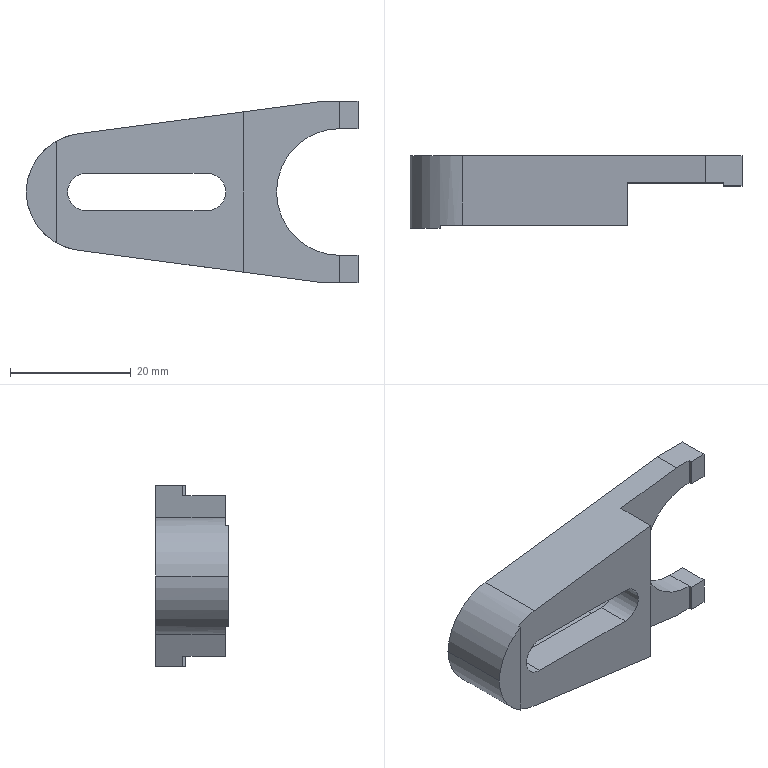Part | SolidWorks | features ICE 4, Extrusion 1, Fillet 1 | 1 solid | 33 faces | box 54.997 x 12 x 30 mm | volume 7361 mm3 | plane 23 | cylinder 10 | commonest cylinder face diameters 6.2 x3 11 x3 20 x2 21 x2
STEP:
#1=CARTESIAN_POINT('',(-50.5,-6.,15.));
#2=VERTEX_POINT('',#1);
#3=CARTESIAN_POINT('',(-45.,-6.,20.5));
#4=VERTEX_POINT('',#3);
#5=CARTESIAN_POINT('',(-45.,-6.,15.));
#6=DIRECTION('',(0.,1.,0.));
#7=DIRECTION('',(-1.,0.,0.));
#8=AXIS2_PLACEMENT_3D('',#5,#6,#7);
#9=CIRCLE('',#8,5.5);
#10=EDGE_CURVE('',#2,#4,#9,.T.);
#11=ORIENTED_EDGE('',*,*,#10,.F.);
#12=CARTESIAN_POINT('',(-50.5,0.,15.));
#13=VERTEX_POINT('',#12);
#14=CARTESIAN_POINT('',(-50.5,-6.,15.));
#15=DIRECTION('',(0.,1.,0.));
#16=VECTOR('',#15,1000.);
#17=LINE('',#14,#16);
#18=EDGE_CURVE('',#2,#13,#17,.T.);
#19=ORIENTED_EDGE('',*,*,#18,.T.);
#20=CARTESIAN_POINT('',(-45.,0.,20.5));
#21=VERTEX_POINT('',#20);
#22=CARTESIAN_POINT('',(-45.,0.,15.));
#23=DIRECTION('',(0.,1.,0.));
#24=DIRECTION('',(-1.,0.,0.));
#25=AXIS2_PLACEMENT_3D('',#22,#23,#24);
#26=CIRCLE('',#25,5.5);
#27=EDGE_CURVE('',#13,#21,#26,.T.);
#28=ORIENTED_EDGE('',*,*,#27,.T.);
#29=CARTESIAN_POINT('',(-45.,-6.,20.5));
#30=DIRECTION('',(0.,1.,0.));
#31=VECTOR('',#30,1000.);
#32=LINE('',#29,#31);
#33=EDGE_CURVE('',#4,#21,#32,.T.);
#34=ORIENTED_EDGE('',*,*,#33,.F.);
#35=EDGE_LOOP('',(#11,#19,#28,#34));
#36=FACE_OUTER_BOUND('',#35,.T.);
#37=CARTESIAN_POINT('',(-45.,-6.,15.));
#38=DIRECTION('',(0.,1.,0.));
#39=DIRECTION('',(-1.,0.,0.));
#40=AXIS2_PLACEMENT_3D('',#37,#38,#39);
#41=CYLINDRICAL_SURFACE('',#40,5.5);
#42=ADVANCED_FACE('',(#36),#41,.F.);
#43=CARTESIAN_POINT('',(-13.5,-4.5,15.));
#44=VERTEX_POINT('',#43);
#45=CARTESIAN_POINT('',(-3.,-4.5,25.5));
#46=VERTEX_POINT('',#45);
#47=CARTESIAN_POINT('',(-3.,-4.5,15.));
#48=DIRECTION('',(0.,1.,0.));
#49=DIRECTION('',(-1.,0.,0.));
#50=AXIS2_PLACEMENT_3D('',#47,#48,#49);
#51=CIRCLE('',#50,10.5);
#52=EDGE_CURVE('',#44,#46,#51,.T.);
#53=ORIENTED_EDGE('',*,*,#52,.F.);
#54=CARTESIAN_POINT('',(-13.5,0.,15.));
#55=VERTEX_POINT('',#54);
#56=CARTESIAN_POINT('',(-13.5,-12.,15.));
#57=DIRECTION('',(0.,1.,0.));
#58=VECTOR('',#57,1000.);
#59=LINE('',#56,#58);
#60=EDGE_CURVE('',#44,#55,#59,.T.);
#61=ORIENTED_EDGE('',*,*,#60,.T.);
#62=CARTESIAN_POINT('',(-3.,0.,25.5));
#63=VERTEX_POINT('',#62);
#64=CARTESIAN_POINT('',(-3.,0.,15.));
#65=DIRECTION('',(0.,1.,0.));
#66=DIRECTION('',(-1.,0.,0.));
#67=AXIS2_PLACEMENT_3D('',#64,#65,#66);
#68=CIRCLE('',#67,10.5);
#69=EDGE_CURVE('',#55,#63,#68,.T.);
#70=ORIENTED_EDGE('',*,*,#69,.T.);
#71=CARTESIAN_POINT('',(-3.,-12.,25.5));
#72=DIRECTION('',(0.,1.,0.));
#73=VECTOR('',#72,1000.);
#74=LINE('',#71,#73);
#75=EDGE_CURVE('',#46,#63,#74,.T.);
#76=ORIENTED_EDGE('',*,*,#75,.F.);
#77=EDGE_LOOP('',(#53,#61,#70,#76));
#78=FACE_OUTER_BOUND('',#77,.T.);
#79=CARTESIAN_POINT('',(-3.,-12.,15.));
#80=DIRECTION('',(0.,1.,0.));
#81=DIRECTION('',(-1.,0.,0.));
#82=AXIS2_PLACEMENT_3D('',#79,#80,#81);
#83=CYLINDRICAL_SURFACE('',#82,10.5);
#84=ADVANCED_FACE('',(#78),#83,.F.);
#85=CARTESIAN_POINT('',(-48.1,-11.5,15.));
#86=VERTEX_POINT('',#85);
#87=CARTESIAN_POINT('',(-45.,-11.5,18.1));
#88=VERTEX_POINT('',#87);
#89=CARTESIAN_POINT('',(-45.,-11.5,15.));
#90=DIRECTION('',(0.,1.,0.));
#91=DIRECTION('',(0.,0.,1.));
#92=AXIS2_PLACEMENT_3D('',#89,#90,#91);
#93=CIRCLE('',#92,3.1);
#94=EDGE_CURVE('',#86,#88,#93,.T.);
#95=ORIENTED_EDGE('',*,*,#94,.F.);
#96=CARTESIAN_POINT('',(-48.1,-6.,15.));
#97=VERTEX_POINT('',#96);
#98=CARTESIAN_POINT('',(-48.1,-12.,15.));
#99=DIRECTION('',(0.,1.,0.));
#100=VECTOR('',#99,1000.);
#101=LINE('',#98,#100);
#102=EDGE_CURVE('',#86,#97,#101,.T.);
#103=ORIENTED_EDGE('',*,*,#102,.T.);
#104=CARTESIAN_POINT('',(-45.,-6.,18.1));
#105=VERTEX_POINT('',#104);
#106=CARTESIAN_POINT('',(-45.,-6.,15.));
#107=DIRECTION('',(0.,-1.,0.));
#108=DIRECTION('',(-1.,0.,0.));
#109=AXIS2_PLACEMENT_3D('',#106,#107,#108);
#110=CIRCLE('',#109,3.1);
#111=EDGE_CURVE('',#105,#97,#110,.T.);
#112=ORIENTED_EDGE('',*,*,#111,.F.);
#113=CARTESIAN_POINT('',(-45.,-12.,18.1));
#114=DIRECTION('',(0.,1.,0.));
#115=VECTOR('',#114,1000.);
#116=LINE('',#113,#115);
#117=EDGE_CURVE('',#88,#105,#116,.T.);
#118=ORIENTED_EDGE('',*,*,#117,.F.);
#119=EDGE_LOOP('',(#95,#103,#112,#118));
#120=FACE_OUTER_BOUND('',#119,.T.);
#121=CARTESIAN_POINT('',(-45.,-12.,15.));
#122=DIRECTION('',(0.,1.,0.));
#123=DIRECTION('',(-1.,0.,0.));
#124=AXIS2_PLACEMENT_3D('',#121,#122,#123);
#125=CYLINDRICAL_SURFACE('',#124,3.1);
#126=ADVANCED_FACE('',(#120),#125,.F.);
#127=ORIENTED_EDGE('',*,*,#102,.F.);
#128=CARTESIAN_POINT('',(-45.,-11.5,11.9));
#129=VERTEX_POINT('',#128);
#130=CARTESIAN_POINT('',(-45.,-11.5,15.));
#131=DIRECTION('',(0.,1.,0.));
#132=DIRECTION('',(0.,0.,1.));
#133=AXIS2_PLACEMENT_3D('',#130,#131,#132);
#134=CIRCLE('',#133,3.1);
#135=EDGE_CURVE('',#129,#86,#134,.T.);
#136=ORIENTED_EDGE('',*,*,#135,.F.);
#137=CARTESIAN_POINT('',(-45.,-6.,11.9));
#138=VERTEX_POINT('',#137);
#139=CARTESIAN_POINT('',(-45.,-12.,11.9));
#140=DIRECTION('',(0.,1.,0.));
#141=VECTOR('',#140,1000.);
#142=LINE('',#139,#141);
#143=EDGE_CURVE('',#129,#138,#142,.T.);
#144=ORIENTED_EDGE('',*,*,#143,.T.);
#145=CARTESIAN_POINT('',(-45.,-6.,15.));
#146=DIRECTION('',(0.,-1.,0.));
#147=DIRECTION('',(-1.,0.,0.));
#148=AXIS2_PLACEMENT_3D('',#145,#146,#147);
#149=CIRCLE('',#148,3.1);
#150=EDGE_CURVE('',#97,#138,#149,.T.);
#151=ORIENTED_EDGE('',*,*,#150,.F.);
#152=EDGE_LOOP('',(#127,#136,#144,#151));
#153=FACE_OUTER_BOUND('',#152,.T.);
#154=CARTESIAN_POINT('',(-45.,-12.,15.));
#155=DIRECTION('',(0.,1.,0.));
#156=DIRECTION('',(-1.,0.,0.));
#157=AXIS2_PLACEMENT_3D('',#154,#155,#156);
#158=CYLINDRICAL_SURFACE('',#157,3.1);
#159=ADVANCED_FACE('',(#153),#158,.F.);
#160=CARTESIAN_POINT('',(-25.,-6.,11.9));
#161=VERTEX_POINT('',#160);
#162=CARTESIAN_POINT('',(-45.,-6.,11.9));
#163=DIRECTION('',(1.,0.,0.));
#164=VECTOR('',#163,1000.);
#165=LINE('',#162,#164);
#166=EDGE_CURVE('',#138,#161,#165,.T.);
#167=ORIENTED_EDGE('',*,*,#166,.F.);
#168=ORIENTED_EDGE('',*,*,#143,.F.);
#169=CARTESIAN_POINT('',(-25.,-11.5,11.9));
#170=VERTEX_POINT('',#169);
#171=CARTESIAN_POINT('',(-50.,-11.5,11.9));
#172=DIRECTION('',(-1.,0.,0.));
#173=VECTOR('',#172,1000.);
#174=LINE('',#171,#173);
#175=EDGE_CURVE('',#170,#129,#174,.T.);
#176=ORIENTED_EDGE('',*,*,#175,.F.);
#177=CARTESIAN_POINT('',(-25.,-12.,11.9));
#178=DIRECTION('',(0.,1.,0.));
#179=VECTOR('',#178,1000.);
#180=LINE('',#177,#179);
#181=EDGE_CURVE('',#170,#161,#180,.T.);
#182=ORIENTED_EDGE('',*,*,#181,.T.);
#183=EDGE_LOOP('',(#167,#168,#176,#182));
#184=FACE_OUTER_BOUND('',#183,.T.);
#185=CARTESIAN_POINT('',(-45.,-12.,11.9));
#186=DIRECTION('',(0.,0.,-1.));
#187=DIRECTION('',(-1.,0.,0.));
#188=AXIS2_PLACEMENT_3D('',#185,#186,#187);
#189=PLANE('',#188);
#190=ADVANCED_FACE('',(#184),#189,.F.);
#191=CARTESIAN_POINT('',(-25.,-6.,18.1));
#192=VERTEX_POINT('',#191);
#193=CARTESIAN_POINT('',(-25.,-6.,15.));
#194=DIRECTION('',(0.,-1.,0.));
#195=DIRECTION('',(-1.,0.,0.));
#196=AXIS2_PLACEMENT_3D('',#193,#194,#195);
#197=CIRCLE('',#196,3.1);
#198=EDGE_CURVE('',#161,#192,#197,.T.);
#199=ORIENTED_EDGE('',*,*,#198,.F.);
#200=ORIENTED_EDGE('',*,*,#181,.F.);
#201=CARTESIAN_POINT('',(-25.,-11.5,18.1));
#202=VERTEX_POINT('',#201);
#203=CARTESIAN_POINT('',(-25.,-11.5,15.));
#204=DIRECTION('',(0.,1.,0.));
#205=DIRECTION('',(0.,0.,1.));
#206=AXIS2_PLACEMENT_3D('',#203,#204,#205);
#207=CIRCLE('',#206,3.1);
#208=EDGE_CURVE('',#202,#170,#207,.T.);
#209=ORIENTED_EDGE('',*,*,#208,.F.);
#210=CARTESIAN_POINT('',(-25.,-12.,18.1));
#211=DIRECTION('',(0.,1.,0.));
#212=VECTOR('',#211,1000.);
#213=LINE('',#210,#212);
#214=EDGE_CURVE('',#202,#192,#213,.T.);
#215=ORIENTED_EDGE('',*,*,#214,.T.);
#216=EDGE_LOOP('',(#199,#200,#209,#215));
#217=FACE_OUTER_BOUND('',#216,.T.);
#218=CARTESIAN_POINT('',(-25.,-12.,15.));
#219=DIRECTION('',(0.,1.,0.));
#220=DIRECTION('',(-1.,0.,0.));
#221=AXIS2_PLACEMENT_3D('',#218,#219,#220);
#222=CYLINDRICAL_SURFACE('',#221,3.1);
#223=ADVANCED_FACE('',(#217),#222,.F.);
#224=CARTESIAN_POINT('',(-45.,-6.,18.1));
#225=DIRECTION('',(-1.,0.,0.));
#226=VECTOR('',#225,1000.);
#227=LINE('',#224,#226);
#228=EDGE_CURVE('',#192,#105,#227,.T.);
#229=ORIENTED_EDGE('',*,*,#228,.F.);
#230=ORIENTED_EDGE('',*,*,#214,.F.);
#231=CARTESIAN_POINT('',(-50.,-11.5,18.1));
#232=DIRECTION('',(1.,0.,0.));
#233=VECTOR('',#232,1000.);
#234=LINE('',#231,#233);
#235=EDGE_CURVE('',#88,#202,#234,.T.);
#236=ORIENTED_EDGE('',*,*,#235,.F.);
#237=ORIENTED_EDGE('',*,*,#117,.T.);
#238=EDGE_LOOP('',(#229,#230,#236,#237));
#239=FACE_OUTER_BOUND('',#238,.T.);
#240=CARTESIAN_POINT('',(-45.,-12.,18.1));
#241=DIRECTION('',(0.,0.,1.));
#242=DIRECTION('',(1.,0.,0.));
#243=AXIS2_PLACEMENT_3D('',#240,#241,#242);
#244=PLANE('',#243);
#245=ADVANCED_FACE('',(#239),#244,.F.);
#246=CARTESIAN_POINT('',(-3.,-4.5,4.5));
#247=VERTEX_POINT('',#246);
#248=CARTESIAN_POINT('',(-3.,-4.5,0.));
#249=VERTEX_POINT('',#248);
#250=CARTESIAN_POINT('',(-3.,-4.5,4.5));
#251=DIRECTION('',(0.,0.,-1.));
#252=VECTOR('',#251,1000.);
#253=LINE('',#250,#252);
#254=EDGE_CURVE('',#247,#249,#253,.T.);
#255=ORIENTED_EDGE('',*,*,#254,.F.);
#256=CARTESIAN_POINT('',(-3.,-4.5,15.));
#257=DIRECTION('',(0.,1.,0.));
#258=DIRECTION('',(-1.,0.,0.));
#259=AXIS2_PLACEMENT_3D('',#256,#257,#258);
#260=CIRCLE('',#259,10.5);
#261=EDGE_CURVE('',#247,#44,#260,.T.);
#262=ORIENTED_EDGE('',*,*,#261,.T.);
#263=ORIENTED_EDGE('',*,*,#52,.T.);
#264=CARTESIAN_POINT('',(-3.,-4.5,30.));
#265=VERTEX_POINT('',#264);
#266=CARTESIAN_POINT('',(-3.,-4.5,25.5));
#267=DIRECTION('',(0.,0.,-1.));
#268=VECTOR('',#267,1000.);
#269=LINE('',#266,#268);
#270=EDGE_CURVE('',#265,#46,#269,.T.);
#271=ORIENTED_EDGE('',*,*,#270,.F.);
#272=CARTESIAN_POINT('',(-6.,-4.5,30.));
#273=VERTEX_POINT('',#272);
#274=CARTESIAN_POINT('',(0.,-4.5,30.));
#275=DIRECTION('',(1.,0.,0.));
#276=VECTOR('',#275,1000.);
#277=LINE('',#274,#276);
#278=EDGE_CURVE('',#273,#265,#277,.T.);
#279=ORIENTED_EDGE('',*,*,#278,.F.);
#280=CARTESIAN_POINT('',(-19.,-4.5,28.276));
#281=VERTEX_POINT('',#280);
#282=CARTESIAN_POINT('',(-0.1038,-4.5,30.782));
#283=DIRECTION('',(-0.9913,0.,-0.1315));
#284=VECTOR('',#283,1000.);
#285=LINE('',#282,#284);
#286=EDGE_CURVE('',#273,#281,#285,.T.);
#287=ORIENTED_EDGE('',*,*,#286,.T.);
#288=CARTESIAN_POINT('',(-19.,-4.5,1.724));
#289=VERTEX_POINT('',#288);
#290=CARTESIAN_POINT('',(-19.,-4.5,30.));
#291=DIRECTION('',(0.,0.,-1.));
#292=VECTOR('',#291,1000.);
#293=LINE('',#290,#292);
#294=EDGE_CURVE('',#281,#289,#293,.T.);
#295=ORIENTED_EDGE('',*,*,#294,.T.);
#296=CARTESIAN_POINT('',(-6.,-4.5,0.));
#297=VERTEX_POINT('',#296);
#298=CARTESIAN_POINT('',(-4.015,-4.5,-0.2634));
#299=DIRECTION('',(0.9913,0.,-0.1315));
#300=VECTOR('',#299,1000.);
#301=LINE('',#298,#300);
#302=EDGE_CURVE('',#289,#297,#301,.T.);
#303=ORIENTED_EDGE('',*,*,#302,.T.);
#304=CARTESIAN_POINT('',(0.,-4.5,0.));
#305=DIRECTION('',(1.,0.,0.));
#306=VECTOR('',#305,1000.);
#307=LINE('',#304,#306);
#308=EDGE_CURVE('',#297,#249,#307,.T.);
#309=ORIENTED_EDGE('',*,*,#308,.T.);
#310=EDGE_LOOP('',(#255,#262,#263,#271,#279,#287,#295,#303,#309));
#311=FACE_OUTER_BOUND('',#310,.T.);
#312=CARTESIAN_POINT('',(0.,-4.5,30.));
#313=DIRECTION('',(0.,1.,0.));
#314=DIRECTION('',(-1.,0.,0.));
#315=AXIS2_PLACEMENT_3D('',#312,#313,#314);
#316=PLANE('',#315);
#317=ADVANCED_FACE('',(#311),#316,.F.);
#318=CARTESIAN_POINT('',(0.,-5.,30.));
#319=VERTEX_POINT('',#318);
#320=CARTESIAN_POINT('',(0.,0.,30.));
#321=VERTEX_POINT('',#320);
#322=CARTESIAN_POINT('',(0.,0.,30.));
#323=DIRECTION('',(0.,1.,0.));
#324=VECTOR('',#323,1000.);
#325=LINE('',#322,#324);
#326=EDGE_CURVE('',#319,#321,#325,.T.);
#327=ORIENTED_EDGE('',*,*,#326,.F.);
#328=CARTESIAN_POINT('',(0.,-5.,25.5));
#329=VERTEX_POINT('',#328);
#330=CARTESIAN_POINT('',(0.,-5.,25.5));
#331=DIRECTION('',(0.,0.,1.));
#332=VECTOR('',#331,1000.);
#333=LINE('',#330,#332);
#334=EDGE_CURVE('',#329,#319,#333,.T.);
#335=ORIENTED_EDGE('',*,*,#334,.F.);
#336=CARTESIAN_POINT('',(0.,0.,25.5));
#337=VERTEX_POINT('',#336);
#338=CARTESIAN_POINT('',(0.,0.,25.5));
#339=DIRECTION('',(0.,1.,0.));
#340=VECTOR('',#339,1000.);
#341=LINE('',#338,#340);
#342=EDGE_CURVE('',#329,#337,#341,.T.);
#343=ORIENTED_EDGE('',*,*,#342,.T.);
#344=CARTESIAN_POINT('',(0.,0.,30.));
#345=DIRECTION('',(0.,0.,-1.));
#346=VECTOR('',#345,1000.);
#347=LINE('',#344,#346);
#348=EDGE_CURVE('',#321,#337,#347,.T.);
#349=ORIENTED_EDGE('',*,*,#348,.F.);
#350=EDGE_LOOP('',(#327,#335,#343,#349));
#351=FACE_OUTER_BOUND('',#350,.T.);
#352=CARTESIAN_POINT('',(0.,0.,30.));
#353=DIRECTION('',(-1.,0.,0.));
#354=DIRECTION('',(0.,-1.,0.));
#355=AXIS2_PLACEMENT_3D('',#352,#353,#354);
#356=PLANE('',#355);
#357=ADVANCED_FACE('',(#351),#356,.F.);
#358=CARTESIAN_POINT('',(0.,0.,4.5));
#359=VERTEX_POINT('',#358);
#360=CARTESIAN_POINT('',(0.,0.,0.));
#361=VERTEX_POINT('',#360);
#362=CARTESIAN_POINT('',(0.,0.,30.));
#363=DIRECTION('',(0.,0.,-1.));
#364=VECTOR('',#363,1000.);
#365=LINE('',#362,#364);
#366=EDGE_CURVE('',#359,#361,#365,.T.);
#367=ORIENTED_EDGE('',*,*,#366,.F.);
#368=CARTESIAN_POINT('',(0.,-5.,4.5));
#369=VERTEX_POINT('',#368);
#370=CARTESIAN_POINT('',(0.,0.,4.5));
#371=DIRECTION('',(0.,-1.,0.));
#372=VECTOR('',#371,1000.);
#373=LINE('',#370,#372);
#374=EDGE_CURVE('',#359,#369,#373,.T.);
#375=ORIENTED_EDGE('',*,*,#374,.T.);
#376=CARTESIAN_POINT('',(0.,-5.,0.));
#377=VERTEX_POINT('',#376);
#378=CARTESIAN_POINT('',(0.,-5.,4.5));
#379=DIRECTION('',(0.,0.,1.));
#380=VECTOR('',#379,1000.);
#381=LINE('',#378,#380);
#382=EDGE_CURVE('',#377,#369,#381,.T.);
#383=ORIENTED_EDGE('',*,*,#382,.F.);
#384=CARTESIAN_POINT('',(0.,0.,0.));
#385=DIRECTION('',(0.,1.,0.));
#386=VECTOR('',#385,1000.);
#387=LINE('',#384,#386);
#388=EDGE_CURVE('',#377,#361,#387,.T.);
#389=ORIENTED_EDGE('',*,*,#388,.T.);
#390=EDGE_LOOP('',(#367,#375,#383,#389));
#391=FACE_OUTER_BOUND('',#390,.T.);
#392=CARTESIAN_POINT('',(0.,0.,30.));
#393=DIRECTION('',(-1.,0.,0.));
#394=DIRECTION('',(0.,-1.,0.));
#395=AXIS2_PLACEMENT_3D('',#392,#393,#394);
#396=PLANE('',#395);
#397=ADVANCED_FACE('',(#391),#396,.F.);
#398=CARTESIAN_POINT('',(-25.,0.,20.5));
#399=VERTEX_POINT('',#398);
#400=CARTESIAN_POINT('',(-45.,0.,20.5));
#401=DIRECTION('',(1.,0.,0.));
#402=VECTOR('',#401,1000.);
#403=LINE('',#400,#402);
#404=EDGE_CURVE('',#21,#399,#403,.T.);
#405=ORIENTED_EDGE('',*,*,#404,.F.);
#406=ORIENTED_EDGE('',*,*,#27,.F.);
#407=CARTESIAN_POINT('',(-45.,0.,9.5));
#408=VERTEX_POINT('',#407);
#409=CARTESIAN_POINT('',(-45.,0.,15.));
#410=DIRECTION('',(0.,1.,0.));
#411=DIRECTION('',(-1.,0.,0.));
#412=AXIS2_PLACEMENT_3D('',#409,#410,#411);
#413=CIRCLE('',#412,5.5);
#414=EDGE_CURVE('',#408,#13,#413,.T.);
#415=ORIENTED_EDGE('',*,*,#414,.F.);
#416=CARTESIAN_POINT('',(-25.,0.,9.5));
#417=VERTEX_POINT('',#416);
#418=CARTESIAN_POINT('',(-45.,0.,9.5));
#419=DIRECTION('',(-1.,0.,0.));
#420=VECTOR('',#419,1000.);
#421=LINE('',#418,#420);
#422=EDGE_CURVE('',#417,#408,#421,.T.);
#423=ORIENTED_EDGE('',*,*,#422,.F.);
#424=CARTESIAN_POINT('',(-25.,0.,15.));
#425=DIRECTION('',(0.,1.,0.));
#426=DIRECTION('',(-1.,0.,0.));
#427=AXIS2_PLACEMENT_3D('',#424,#425,#426);
#428=CIRCLE('',#427,5.5);
#429=EDGE_CURVE('',#399,#417,#428,.T.);
#430=ORIENTED_EDGE('',*,*,#429,.F.);
#431=EDGE_LOOP('',(#405,#406,#415,#423,#430));
#432=FACE_BOUND('',#431,.T.);
#433=CARTESIAN_POINT('',(-46.315,0.,5.348));
#434=VERTEX_POINT('',#433);
#435=CARTESIAN_POINT('',(-6.,0.,0.));
#436=VERTEX_POINT('',#435);
#437=CARTESIAN_POINT('',(-6.,0.,0.));
#438=DIRECTION('',(0.9913,0.,-0.1315));
#439=VECTOR('',#438,1000.);
#440=LINE('',#437,#439);
#441=EDGE_CURVE('',#434,#436,#440,.T.);
#442=ORIENTED_EDGE('',*,*,#441,.F.);
#443=CARTESIAN_POINT('',(-54.997,0.,15.));
#444=VERTEX_POINT('',#443);
#445=CARTESIAN_POINT('',(-45.,0.,15.261));
#446=DIRECTION('',(0.,1.,0.));
#447=DIRECTION('',(1.,0.,0.));
#448=AXIS2_PLACEMENT_3D('',#445,#446,#447);
#449=CIRCLE('',#448,10.);
#450=EDGE_CURVE('',#434,#444,#449,.T.);
#451=ORIENTED_EDGE('',*,*,#450,.T.);
#452=CARTESIAN_POINT('',(-46.315,0.,24.652));
#453=VERTEX_POINT('',#452);
#454=CARTESIAN_POINT('',(-45.,0.,14.739));
#455=DIRECTION('',(0.,1.,0.));
#456=DIRECTION('',(1.,0.,0.));
#457=AXIS2_PLACEMENT_3D('',#454,#455,#456);
#458=CIRCLE('',#457,10.);
#459=EDGE_CURVE('',#444,#453,#458,.T.);
#460=ORIENTED_EDGE('',*,*,#459,.T.);
#461=CARTESIAN_POINT('',(-6.,0.,30.));
#462=VERTEX_POINT('',#461);
#463=CARTESIAN_POINT('',(-55.,0.,23.5));
#464=DIRECTION('',(-0.9913,0.,-0.1315));
#465=VECTOR('',#464,1000.);
#466=LINE('',#463,#465);
#467=EDGE_CURVE('',#462,#453,#466,.T.);
#468=ORIENTED_EDGE('',*,*,#467,.F.);
#469=CARTESIAN_POINT('',(0.,0.,30.));
#470=DIRECTION('',(-1.,0.,0.));
#471=VECTOR('',#470,1000.);
#472=LINE('',#469,#471);
#473=EDGE_CURVE('',#321,#462,#472,.T.);
#474=ORIENTED_EDGE('',*,*,#473,.F.);
#475=ORIENTED_EDGE('',*,*,#348,.T.);
#476=CARTESIAN_POINT('',(3.,0.,25.5));
#477=DIRECTION('',(1.,0.,0.));
#478=VECTOR('',#477,1000.);
#479=LINE('',#476,#478);
#480=EDGE_CURVE('',#63,#337,#479,.T.);
#481=ORIENTED_EDGE('',*,*,#480,.F.);
#482=ORIENTED_EDGE('',*,*,#69,.F.);
#483=CARTESIAN_POINT('',(-3.,0.,4.5));
#484=VERTEX_POINT('',#483);
#485=CARTESIAN_POINT('',(-3.,0.,15.));
#486=DIRECTION('',(0.,1.,0.));
#487=DIRECTION('',(-1.,0.,0.));
#488=AXIS2_PLACEMENT_3D('',#485,#486,#487);
#489=CIRCLE('',#488,10.5);
#490=EDGE_CURVE('',#484,#55,#489,.T.);
#491=ORIENTED_EDGE('',*,*,#490,.F.);
#492=CARTESIAN_POINT('',(3.,0.,4.5));
#493=DIRECTION('',(-1.,0.,0.));
#494=VECTOR('',#493,1000.);
#495=LINE('',#492,#494);
#496=EDGE_CURVE('',#359,#484,#495,.T.);
#497=ORIENTED_EDGE('',*,*,#496,.F.);
#498=ORIENTED_EDGE('',*,*,#366,.T.);
#499=CARTESIAN_POINT('',(0.,0.,0.));
#500=DIRECTION('',(-1.,0.,0.));
#501=VECTOR('',#500,1000.);
#502=LINE('',#499,#501);
#503=EDGE_CURVE('',#361,#436,#502,.T.);
#504=ORIENTED_EDGE('',*,*,#503,.T.);
#505=EDGE_LOOP('',(#442,#451,#460,#468,#474,#475,#481,#482,#491,#497,#498,#504));
#506=FACE_OUTER_BOUND('',#505,.T.);
#507=CARTESIAN_POINT('',(0.,0.,30.));
#508=DIRECTION('',(0.,-1.,0.));
#509=DIRECTION('',(1.,0.,0.));
#510=AXIS2_PLACEMENT_3D('',#507,#508,#509);
#511=PLANE('',#510);
#512=ADVANCED_FACE('',(#432,#506),#511,.F.);
#513=CARTESIAN_POINT('',(-50.,-12.,23.399));
#514=VERTEX_POINT('',#513);
#515=CARTESIAN_POINT('',(-54.997,-12.,15.));
#516=VERTEX_POINT('',#515);
#517=CARTESIAN_POINT('',(-45.,-12.,14.739));
#518=DIRECTION('',(0.,-1.,0.));
#519=DIRECTION('',(-1.,0.,0.));
#520=AXIS2_PLACEMENT_3D('',#517,#518,#519);
#521=CIRCLE('',#520,10.);
#522=EDGE_CURVE('',#514,#516,#521,.T.);
#523=ORIENTED_EDGE('',*,*,#522,.T.);
#524=CARTESIAN_POINT('',(-50.,-12.,6.601));
#525=VERTEX_POINT('',#524);
#526=CARTESIAN_POINT('',(-45.,-12.,15.261));
#527=DIRECTION('',(0.,-1.,0.));
#528=DIRECTION('',(-1.,0.,0.));
#529=AXIS2_PLACEMENT_3D('',#526,#527,#528);
#530=CIRCLE('',#529,10.);
#531=EDGE_CURVE('',#516,#525,#530,.T.);
#532=ORIENTED_EDGE('',*,*,#531,.T.);
#533=CARTESIAN_POINT('',(-50.,-12.,30.));
#534=DIRECTION('',(0.,0.,-1.));
#535=VECTOR('',#534,1000.);
#536=LINE('',#533,#535);
#537=EDGE_CURVE('',#514,#525,#536,.T.);
#538=ORIENTED_EDGE('',*,*,#537,.F.);
#539=EDGE_LOOP('',(#523,#532,#538));
#540=FACE_OUTER_BOUND('',#539,.T.);
#541=CARTESIAN_POINT('',(-55.,-12.,30.));
#542=DIRECTION('',(0.,1.,0.));
#543=DIRECTION('',(-1.,0.,0.));
#544=AXIS2_PLACEMENT_3D('',#541,#542,#543);
#545=PLANE('',#544);
#546=ADVANCED_FACE('',(#540),#545,.F.);
#547=ORIENTED_EDGE('',*,*,#537,.T.);
#548=CARTESIAN_POINT('',(-50.,-11.5,6.601));
#549=VERTEX_POINT('',#548);
#550=CARTESIAN_POINT('',(-50.,-12.,6.601));
#551=DIRECTION('',(0.,1.,0.));
#552=VECTOR('',#551,1000.);
#553=LINE('',#550,#552);
#554=EDGE_CURVE('',#525,#549,#553,.T.);
#555=ORIENTED_EDGE('',*,*,#554,.T.);
#556=CARTESIAN_POINT('',(-50.,-11.5,23.399));
#557=VERTEX_POINT('',#556);
#558=CARTESIAN_POINT('',(-50.,-11.5,30.));
#559=DIRECTION('',(0.,0.,-1.));
#560=VECTOR('',#559,1000.);
#561=LINE('',#558,#560);
#562=EDGE_CURVE('',#557,#549,#561,.T.);
#563=ORIENTED_EDGE('',*,*,#562,.F.);
#564=CARTESIAN_POINT('',(-50.,-11.5,23.399));
#565=DIRECTION('',(0.,-1.,0.));
#566=VECTOR('',#565,1000.);
#567=LINE('',#564,#566);
#568=EDGE_CURVE('',#557,#514,#567,.T.);
#569=ORIENTED_EDGE('',*,*,#568,.T.);
#570=EDGE_LOOP('',(#547,#555,#563,#569));
#571=FACE_OUTER_BOUND('',#570,.T.);
#572=CARTESIAN_POINT('',(-50.,-12.,30.));
#573=DIRECTION('',(-1.,0.,0.));
#574=DIRECTION('',(0.,0.,1.));
#575=AXIS2_PLACEMENT_3D('',#572,#573,#574);
#576=PLANE('',#575);
#577=ADVANCED_FACE('',(#571),#576,.F.);
#578=ORIENTED_EDGE('',*,*,#175,.T.);
#579=ORIENTED_EDGE('',*,*,#135,.T.);
#580=ORIENTED_EDGE('',*,*,#94,.T.);
#581=ORIENTED_EDGE('',*,*,#235,.T.);
#582=ORIENTED_EDGE('',*,*,#208,.T.);
#583=EDGE_LOOP('',(#578,#579,#580,#581,#582));
#584=FACE_BOUND('',#583,.T.);
#585=ORIENTED_EDGE('',*,*,#562,.T.);
#586=CARTESIAN_POINT('',(-46.315,-11.5,5.348));
#587=VERTEX_POINT('',#586);
#588=CARTESIAN_POINT('',(-45.,-11.5,15.261));
#589=DIRECTION('',(0.,-1.,0.));
#590=DIRECTION('',(0.,0.,1.));
#591=AXIS2_PLACEMENT_3D('',#588,#589,#590);
#592=CIRCLE('',#591,10.);
#593=EDGE_CURVE('',#549,#587,#592,.T.);
#594=ORIENTED_EDGE('',*,*,#593,.T.);
#595=CARTESIAN_POINT('',(-19.,-11.5,1.724));
#596=VERTEX_POINT('',#595);
#597=CARTESIAN_POINT('',(-53.15,-11.5,6.255));
#598=DIRECTION('',(0.9913,0.,-0.1315));
#599=VECTOR('',#598,1000.);
#600=LINE('',#597,#599);
#601=EDGE_CURVE('',#587,#596,#600,.T.);
#602=ORIENTED_EDGE('',*,*,#601,.T.);
#603=CARTESIAN_POINT('',(-19.,-11.5,28.276));
#604=VERTEX_POINT('',#603);
#605=CARTESIAN_POINT('',(-19.,-11.5,30.));
#606=DIRECTION('',(0.,0.,-1.));
#607=VECTOR('',#606,1000.);
#608=LINE('',#605,#607);
#609=EDGE_CURVE('',#604,#596,#608,.T.);
#610=ORIENTED_EDGE('',*,*,#609,.F.);
#611=CARTESIAN_POINT('',(-46.315,-11.5,24.652));
#612=VERTEX_POINT('',#611);
#613=CARTESIAN_POINT('',(-49.239,-11.5,24.264));
#614=DIRECTION('',(-0.9913,0.,-0.1315));
#615=VECTOR('',#614,1000.);
#616=LINE('',#613,#615);
#617=EDGE_CURVE('',#604,#612,#616,.T.);
#618=ORIENTED_EDGE('',*,*,#617,.T.);
#619=CARTESIAN_POINT('',(-45.,-11.5,14.739));
#620=DIRECTION('',(0.,-1.,0.));
#621=DIRECTION('',(0.,0.,1.));
#622=AXIS2_PLACEMENT_3D('',#619,#620,#621);
#623=CIRCLE('',#622,10.);
#624=EDGE_CURVE('',#612,#557,#623,.T.);
#625=ORIENTED_EDGE('',*,*,#624,.T.);
#626=EDGE_LOOP('',(#585,#594,#602,#610,#618,#625));
#627=FACE_OUTER_BOUND('',#626,.T.);
#628=CARTESIAN_POINT('',(-50.,-11.5,30.));
#629=DIRECTION('',(0.,1.,0.));
#630=DIRECTION('',(0.,0.,1.));
#631=AXIS2_PLACEMENT_3D('',#628,#629,#630);
#632=PLANE('',#631);
#633=ADVANCED_FACE('',(#584,#627),#632,.F.);
#634=ORIENTED_EDGE('',*,*,#294,.F.);
#635=CARTESIAN_POINT('',(-19.,-11.5,28.276));
#636=DIRECTION('',(0.,-1.,0.));
#637=VECTOR('',#636,1000.);
#638=LINE('',#635,#637);
#639=EDGE_CURVE('',#281,#604,#638,.T.);
#640=ORIENTED_EDGE('',*,*,#639,.T.);
#641=ORIENTED_EDGE('',*,*,#609,.T.);
#642=CARTESIAN_POINT('',(-19.,-11.5,1.724));
#643=DIRECTION('',(0.,1.,0.));
#644=VECTOR('',#643,1000.);
#645=LINE('',#642,#644);
#646=EDGE_CURVE('',#596,#289,#645,.T.);
#647=ORIENTED_EDGE('',*,*,#646,.T.);
#648=EDGE_LOOP('',(#634,#640,#641,#647));
#649=FACE_OUTER_BOUND('',#648,.T.);
#650=CARTESIAN_POINT('',(-19.,-11.5,30.));
#651=DIRECTION('',(-1.,0.,0.));
#652=DIRECTION('',(0.,0.,1.));
#653=AXIS2_PLACEMENT_3D('',#650,#651,#652);
#654=PLANE('',#653);
#655=ADVANCED_FACE('',(#649),#654,.F.);
#656=ORIENTED_EDGE('',*,*,#473,.T.);
#657=CARTESIAN_POINT('',(-6.,0.,30.));
#658=DIRECTION('',(0.,-1.,0.));
#659=VECTOR('',#658,1000.);
#660=LINE('',#657,#659);
#661=EDGE_CURVE('',#462,#273,#660,.T.);
#662=ORIENTED_EDGE('',*,*,#661,.T.);
#663=ORIENTED_EDGE('',*,*,#278,.T.);
#664=CARTESIAN_POINT('',(-3.,-5.,30.));
#665=VERTEX_POINT('',#664);
#666=CARTESIAN_POINT('',(-3.,-5.,30.));
#667=DIRECTION('',(0.,1.,0.));
#668=VECTOR('',#667,1000.);
#669=LINE('',#666,#668);
#670=EDGE_CURVE('',#665,#265,#669,.T.);
#671=ORIENTED_EDGE('',*,*,#670,.F.);
#672=CARTESIAN_POINT('',(-3.,-5.,30.));
#673=DIRECTION('',(-1.,0.,0.));
#674=VECTOR('',#673,1000.);
#675=LINE('',#672,#674);
#676=EDGE_CURVE('',#319,#665,#675,.T.);
#677=ORIENTED_EDGE('',*,*,#676,.F.);
#678=ORIENTED_EDGE('',*,*,#326,.T.);
#679=EDGE_LOOP('',(#656,#662,#663,#671,#677,#678));
#680=FACE_OUTER_BOUND('',#679,.T.);
#681=CARTESIAN_POINT('',(0.,0.,30.));
#682=DIRECTION('',(0.,0.,-1.));
#683=DIRECTION('',(-1.,0.,0.));
#684=AXIS2_PLACEMENT_3D('',#681,#682,#683);
#685=PLANE('',#684);
#686=ADVANCED_FACE('',(#680),#685,.F.);
#687=CARTESIAN_POINT('',(-6.,0.,0.));
#688=DIRECTION('',(0.,-1.,0.));
#689=VECTOR('',#688,1000.);
#690=LINE('',#687,#689);
#691=EDGE_CURVE('',#436,#297,#690,.T.);
#692=ORIENTED_EDGE('',*,*,#691,.F.);
#693=ORIENTED_EDGE('',*,*,#503,.F.);
#694=ORIENTED_EDGE('',*,*,#388,.F.);
#695=CARTESIAN_POINT('',(-3.,-5.,0.));
#696=VERTEX_POINT('',#695);
#697=CARTESIAN_POINT('',(0.,-5.,0.));
#698=DIRECTION('',(1.,0.,0.));
#699=VECTOR('',#698,1000.);
#700=LINE('',#697,#699);
#701=EDGE_CURVE('',#696,#377,#700,.T.);
#702=ORIENTED_EDGE('',*,*,#701,.F.);
#703=CARTESIAN_POINT('',(-3.,-5.,0.));
#704=DIRECTION('',(0.,1.,0.));
#705=VECTOR('',#704,1000.);
#706=LINE('',#703,#705);
#707=EDGE_CURVE('',#696,#249,#706,.T.);
#708=ORIENTED_EDGE('',*,*,#707,.T.);
#709=ORIENTED_EDGE('',*,*,#308,.F.);
#710=EDGE_LOOP('',(#692,#693,#694,#702,#708,#709));
#711=FACE_OUTER_BOUND('',#710,.T.);
#712=CARTESIAN_POINT('',(0.,0.,0.));
#713=DIRECTION('',(0.,0.,-1.));
#714=DIRECTION('',(-1.,0.,0.));
#715=AXIS2_PLACEMENT_3D('',#712,#713,#714);
#716=PLANE('',#715);
#717=ADVANCED_FACE('',(#711),#716,.T.);
#718=ORIENTED_EDGE('',*,*,#601,.F.);
#719=CARTESIAN_POINT('',(-46.315,-12.,5.348));
#720=DIRECTION('',(0.,1.,0.));
#721=VECTOR('',#720,1000.);
#722=LINE('',#719,#721);
#723=EDGE_CURVE('',#587,#434,#722,.T.);
#724=ORIENTED_EDGE('',*,*,#723,.T.);
#725=ORIENTED_EDGE('',*,*,#441,.T.);
#726=ORIENTED_EDGE('',*,*,#691,.T.);
#727=ORIENTED_EDGE('',*,*,#302,.F.);
#728=ORIENTED_EDGE('',*,*,#646,.F.);
#729=EDGE_LOOP('',(#718,#724,#725,#726,#727,#728));
#730=FACE_OUTER_BOUND('',#729,.T.);
#731=CARTESIAN_POINT('',(-6.,-12.,0.));
#732=DIRECTION('',(0.1315,0.,0.9913));
#733=DIRECTION('',(0.9913,0.,-0.1315));
#734=AXIS2_PLACEMENT_3D('',#731,#732,#733);
#735=PLANE('',#734);
#736=ADVANCED_FACE('',(#730),#735,.F.);
#737=ORIENTED_EDGE('',*,*,#467,.T.);
#738=CARTESIAN_POINT('',(-46.315,-12.,24.652));
#739=DIRECTION('',(0.,-1.,0.));
#740=VECTOR('',#739,1000.);
#741=LINE('',#738,#740);
#742=EDGE_CURVE('',#453,#612,#741,.T.);
#743=ORIENTED_EDGE('',*,*,#742,.T.);
#744=ORIENTED_EDGE('',*,*,#617,.F.);
#745=ORIENTED_EDGE('',*,*,#639,.F.);
#746=ORIENTED_EDGE('',*,*,#286,.F.);
#747=ORIENTED_EDGE('',*,*,#661,.F.);
#748=EDGE_LOOP('',(#737,#743,#744,#745,#746,#747));
#749=FACE_OUTER_BOUND('',#748,.T.);
#750=CARTESIAN_POINT('',(-55.,-12.,23.5));
#751=DIRECTION('',(0.1315,0.,-0.9913));
#752=DIRECTION('',(-0.9913,0.,-0.1315));
#753=AXIS2_PLACEMENT_3D('',#750,#751,#752);
#754=PLANE('',#753);
#755=ADVANCED_FACE('',(#749),#754,.F.);
#756=ORIENTED_EDGE('',*,*,#342,.F.);
#757=CARTESIAN_POINT('',(-3.,-5.,25.5));
#758=VERTEX_POINT('',#757);
#759=CARTESIAN_POINT('',(-3.,-5.,25.5));
#760=DIRECTION('',(1.,0.,0.));
#761=VECTOR('',#760,1000.);
#762=LINE('',#759,#761);
#763=EDGE_CURVE('',#758,#329,#762,.T.);
#764=ORIENTED_EDGE('',*,*,#763,.F.);
#765=CARTESIAN_POINT('',(-3.,-5.,25.5));
#766=DIRECTION('',(0.,1.,0.));
#767=VECTOR('',#766,1000.);
#768=LINE('',#765,#767);
#769=EDGE_CURVE('',#758,#46,#768,.T.);
#770=ORIENTED_EDGE('',*,*,#769,.T.);
#771=ORIENTED_EDGE('',*,*,#75,.T.);
#772=ORIENTED_EDGE('',*,*,#480,.T.);
#773=EDGE_LOOP('',(#756,#764,#770,#771,#772));
#774=FACE_OUTER_BOUND('',#773,.T.);
#775=CARTESIAN_POINT('',(3.,-12.,25.5));
#776=DIRECTION('',(0.,0.,1.));
#777=DIRECTION('',(1.,0.,0.));
#778=AXIS2_PLACEMENT_3D('',#775,#776,#777);
#779=PLANE('',#778);
#780=ADVANCED_FACE('',(#774),#779,.F.);
#781=ORIENTED_EDGE('',*,*,#60,.F.);
#782=ORIENTED_EDGE('',*,*,#261,.F.);
#783=CARTESIAN_POINT('',(-3.,-12.,4.5));
#784=DIRECTION('',(0.,1.,0.));
#785=VECTOR('',#784,1000.);
#786=LINE('',#783,#785);
#787=EDGE_CURVE('',#247,#484,#786,.T.);
#788=ORIENTED_EDGE('',*,*,#787,.T.);
#789=ORIENTED_EDGE('',*,*,#490,.T.);
#790=EDGE_LOOP('',(#781,#782,#788,#789));
#791=FACE_OUTER_BOUND('',#790,.T.);
#792=CARTESIAN_POINT('',(-3.,-12.,15.));
#793=DIRECTION('',(0.,1.,0.));
#794=DIRECTION('',(-1.,0.,0.));
#795=AXIS2_PLACEMENT_3D('',#792,#793,#794);
#796=CYLINDRICAL_SURFACE('',#795,10.5);
#797=ADVANCED_FACE('',(#791),#796,.F.);
#798=ORIENTED_EDGE('',*,*,#496,.T.);
#799=ORIENTED_EDGE('',*,*,#787,.F.);
#800=CARTESIAN_POINT('',(-3.,-5.,4.5));
#801=VERTEX_POINT('',#800);
#802=CARTESIAN_POINT('',(-3.,-5.,4.5));
#803=DIRECTION('',(0.,1.,0.));
#804=VECTOR('',#803,1000.);
#805=LINE('',#802,#804);
#806=EDGE_CURVE('',#801,#247,#805,.T.);
#807=ORIENTED_EDGE('',*,*,#806,.F.);
#808=CARTESIAN_POINT('',(0.,-5.,4.5));
#809=DIRECTION('',(-1.,0.,0.));
#810=VECTOR('',#809,1000.);
#811=LINE('',#808,#810);
#812=EDGE_CURVE('',#369,#801,#811,.T.);
#813=ORIENTED_EDGE('',*,*,#812,.F.);
#814=ORIENTED_EDGE('',*,*,#374,.F.);
#815=EDGE_LOOP('',(#798,#799,#807,#813,#814));
#816=FACE_OUTER_BOUND('',#815,.T.);
#817=CARTESIAN_POINT('',(3.,-12.,4.5));
#818=DIRECTION('',(0.,0.,-1.));
#819=DIRECTION('',(-1.,0.,0.));
#820=AXIS2_PLACEMENT_3D('',#817,#818,#819);
#821=PLANE('',#820);
#822=ADVANCED_FACE('',(#816),#821,.F.);
#823=ORIENTED_EDGE('',*,*,#270,.T.);
#824=ORIENTED_EDGE('',*,*,#769,.F.);
#825=CARTESIAN_POINT('',(-3.,-5.,25.5));
#826=DIRECTION('',(0.,0.,-1.));
#827=VECTOR('',#826,1000.);
#828=LINE('',#825,#827);
#829=EDGE_CURVE('',#665,#758,#828,.T.);
#830=ORIENTED_EDGE('',*,*,#829,.F.);
#831=ORIENTED_EDGE('',*,*,#670,.T.);
#832=EDGE_LOOP('',(#823,#824,#830,#831));
#833=FACE_OUTER_BOUND('',#832,.T.);
#834=CARTESIAN_POINT('',(-3.,-5.,25.5));
#835=DIRECTION('',(1.,0.,0.));
#836=DIRECTION('',(0.,1.,0.));
#837=AXIS2_PLACEMENT_3D('',#834,#835,#836);
#838=PLANE('',#837);
#839=ADVANCED_FACE('',(#833),#838,.F.);
#840=ORIENTED_EDGE('',*,*,#829,.T.);
#841=ORIENTED_EDGE('',*,*,#763,.T.);
#842=ORIENTED_EDGE('',*,*,#334,.T.);
#843=ORIENTED_EDGE('',*,*,#676,.T.);
#844=EDGE_LOOP('',(#840,#841,#842,#843));
#845=FACE_OUTER_BOUND('',#844,.T.);
#846=CARTESIAN_POINT('',(0.,-5.,0.));
#847=DIRECTION('',(0.,1.,0.));
#848=DIRECTION('',(-1.,0.,0.));
#849=AXIS2_PLACEMENT_3D('',#846,#847,#848);
#850=PLANE('',#849);
#851=ADVANCED_FACE('',(#845),#850,.F.);
#852=ORIENTED_EDGE('',*,*,#254,.T.);
#853=ORIENTED_EDGE('',*,*,#707,.F.);
#854=CARTESIAN_POINT('',(-3.,-5.,4.5));
#855=DIRECTION('',(0.,0.,-1.));
#856=VECTOR('',#855,1000.);
#857=LINE('',#854,#856);
#858=EDGE_CURVE('',#801,#696,#857,.T.);
#859=ORIENTED_EDGE('',*,*,#858,.F.);
#860=ORIENTED_EDGE('',*,*,#806,.T.);
#861=EDGE_LOOP('',(#852,#853,#859,#860));
#862=FACE_OUTER_BOUND('',#861,.T.);
#863=CARTESIAN_POINT('',(-3.,-5.,4.5));
#864=DIRECTION('',(1.,0.,0.));
#865=DIRECTION('',(0.,1.,0.));
#866=AXIS2_PLACEMENT_3D('',#863,#864,#865);
#867=PLANE('',#866);
#868=ADVANCED_FACE('',(#862),#867,.F.);
#869=ORIENTED_EDGE('',*,*,#382,.T.);
#870=ORIENTED_EDGE('',*,*,#812,.T.);
#871=ORIENTED_EDGE('',*,*,#858,.T.);
#872=ORIENTED_EDGE('',*,*,#701,.T.);
#873=EDGE_LOOP('',(#869,#870,#871,#872));
#874=FACE_OUTER_BOUND('',#873,.T.);
#875=CARTESIAN_POINT('',(0.,-5.,0.));
#876=DIRECTION('',(0.,1.,0.));
#877=DIRECTION('',(-1.,0.,0.));
#878=AXIS2_PLACEMENT_3D('',#875,#876,#877);
#879=PLANE('',#878);
#880=ADVANCED_FACE('',(#874),#879,.F.);
#881=CARTESIAN_POINT('',(-54.997,-6.,15.));
#882=DIRECTION('',(0.,1.,0.));
#883=VECTOR('',#882,1000.);
#884=LINE('',#881,#883);
#885=EDGE_CURVE('',#516,#444,#884,.T.);
#886=ORIENTED_EDGE('',*,*,#885,.F.);
#887=ORIENTED_EDGE('',*,*,#522,.F.);
#888=ORIENTED_EDGE('',*,*,#568,.F.);
#889=ORIENTED_EDGE('',*,*,#624,.F.);
#890=ORIENTED_EDGE('',*,*,#742,.F.);
#891=ORIENTED_EDGE('',*,*,#459,.F.);
#892=EDGE_LOOP('',(#886,#887,#888,#889,#890,#891));
#893=FACE_OUTER_BOUND('',#892,.T.);
#894=CARTESIAN_POINT('',(-45.,0.,14.739));
#895=DIRECTION('',(0.,1.,0.));
#896=DIRECTION('',(0.,0.,1.));
#897=AXIS2_PLACEMENT_3D('',#894,#895,#896);
#898=CYLINDRICAL_SURFACE('',#897,10.);
#899=ADVANCED_FACE('',(#893),#898,.T.);
#900=ORIENTED_EDGE('',*,*,#531,.F.);
#901=ORIENTED_EDGE('',*,*,#885,.T.);
#902=ORIENTED_EDGE('',*,*,#450,.F.);
#903=ORIENTED_EDGE('',*,*,#723,.F.);
#904=ORIENTED_EDGE('',*,*,#593,.F.);
#905=ORIENTED_EDGE('',*,*,#554,.F.);
#906=EDGE_LOOP('',(#900,#901,#902,#903,#904,#905));
#907=FACE_OUTER_BOUND('',#906,.T.);
#908=CARTESIAN_POINT('',(-45.,-12.,15.261));
#909=DIRECTION('',(0.,1.,0.));
#910=DIRECTION('',(0.,0.,1.));
#911=AXIS2_PLACEMENT_3D('',#908,#909,#910);
#912=CYLINDRICAL_SURFACE('',#911,10.);
#913=ADVANCED_FACE('',(#907),#912,.T.);
#914=CARTESIAN_POINT('',(-45.,-6.,9.5));
#915=VERTEX_POINT('',#914);
#916=CARTESIAN_POINT('',(-45.,-6.,15.));
#917=DIRECTION('',(0.,1.,0.));
#918=DIRECTION('',(-1.,0.,0.));
#919=AXIS2_PLACEMENT_3D('',#916,#917,#918);
#920=CIRCLE('',#919,5.5);
#921=EDGE_CURVE('',#915,#2,#920,.T.);
#922=ORIENTED_EDGE('',*,*,#921,.T.);
#923=ORIENTED_EDGE('',*,*,#10,.T.);
#924=CARTESIAN_POINT('',(-25.,-6.,20.5));
#925=VERTEX_POINT('',#924);
#926=CARTESIAN_POINT('',(-45.,-6.,20.5));
#927=DIRECTION('',(1.,0.,0.));
#928=VECTOR('',#927,1000.);
#929=LINE('',#926,#928);
#930=EDGE_CURVE('',#4,#925,#929,.T.);
#931=ORIENTED_EDGE('',*,*,#930,.T.);
#932=CARTESIAN_POINT('',(-25.,-6.,9.5));
#933=VERTEX_POINT('',#932);
#934=CARTESIAN_POINT('',(-25.,-6.,15.));
#935=DIRECTION('',(0.,1.,0.));
#936=DIRECTION('',(-1.,0.,0.));
#937=AXIS2_PLACEMENT_3D('',#934,#935,#936);
#938=CIRCLE('',#937,5.5);
#939=EDGE_CURVE('',#925,#933,#938,.T.);
#940=ORIENTED_EDGE('',*,*,#939,.T.);
#941=CARTESIAN_POINT('',(-45.,-6.,9.5));
#942=DIRECTION('',(-1.,0.,0.));
#943=VECTOR('',#942,1000.);
#944=LINE('',#941,#943);
#945=EDGE_CURVE('',#933,#915,#944,.T.);
#946=ORIENTED_EDGE('',*,*,#945,.T.);
#947=EDGE_LOOP('',(#922,#923,#931,#940,#946));
#948=FACE_OUTER_BOUND('',#947,.T.);
#949=ORIENTED_EDGE('',*,*,#111,.T.);
#950=ORIENTED_EDGE('',*,*,#150,.T.);
#951=ORIENTED_EDGE('',*,*,#166,.T.);
#952=ORIENTED_EDGE('',*,*,#198,.T.);
#953=ORIENTED_EDGE('',*,*,#228,.T.);
#954=EDGE_LOOP('',(#949,#950,#951,#952,#953));
#955=FACE_BOUND('',#954,.T.);
#956=CARTESIAN_POINT('',(-45.,-6.,15.));
#957=DIRECTION('',(0.,1.,0.));
#958=DIRECTION('',(-1.,0.,0.));
#959=AXIS2_PLACEMENT_3D('',#956,#957,#958);
#960=PLANE('',#959);
#961=ADVANCED_FACE('',(#948,#955),#960,.T.);
#962=ORIENTED_EDGE('',*,*,#18,.F.);
#963=ORIENTED_EDGE('',*,*,#921,.F.);
#964=CARTESIAN_POINT('',(-45.,-6.,9.5));
#965=DIRECTION('',(0.,1.,0.));
#966=VECTOR('',#965,1000.);
#967=LINE('',#964,#966);
#968=EDGE_CURVE('',#915,#408,#967,.T.);
#969=ORIENTED_EDGE('',*,*,#968,.T.);
#970=ORIENTED_EDGE('',*,*,#414,.T.);
#971=EDGE_LOOP('',(#962,#963,#969,#970));
#972=FACE_OUTER_BOUND('',#971,.T.);
#973=CARTESIAN_POINT('',(-45.,-6.,15.));
#974=DIRECTION('',(0.,1.,0.));
#975=DIRECTION('',(-1.,0.,0.));
#976=AXIS2_PLACEMENT_3D('',#973,#974,#975);
#977=CYLINDRICAL_SURFACE('',#976,5.5);
#978=ADVANCED_FACE('',(#972),#977,.F.);
#979=ORIENTED_EDGE('',*,*,#422,.T.);
#980=ORIENTED_EDGE('',*,*,#968,.F.);
#981=ORIENTED_EDGE('',*,*,#945,.F.);
#982=CARTESIAN_POINT('',(-25.,-6.,9.5));
#983=DIRECTION('',(0.,1.,0.));
#984=VECTOR('',#983,1000.);
#985=LINE('',#982,#984);
#986=EDGE_CURVE('',#933,#417,#985,.T.);
#987=ORIENTED_EDGE('',*,*,#986,.T.);
#988=EDGE_LOOP('',(#979,#980,#981,#987));
#989=FACE_OUTER_BOUND('',#988,.T.);
#990=CARTESIAN_POINT('',(-45.,-6.,9.5));
#991=DIRECTION('',(0.,0.,-1.));
#992=DIRECTION('',(-1.,0.,0.));
#993=AXIS2_PLACEMENT_3D('',#990,#991,#992);
#994=PLANE('',#993);
#995=ADVANCED_FACE('',(#989),#994,.F.);
#996=ORIENTED_EDGE('',*,*,#429,.T.);
#997=ORIENTED_EDGE('',*,*,#986,.F.);
#998=ORIENTED_EDGE('',*,*,#939,.F.);
#999=CARTESIAN_POINT('',(-25.,-6.,20.5));
#1000=DIRECTION('',(0.,1.,0.));
#1001=VECTOR('',#1000,1000.);
#1002=LINE('',#999,#1001);
#1003=EDGE_CURVE('',#925,#399,#1002,.T.);
#1004=ORIENTED_EDGE('',*,*,#1003,.T.);
#1005=EDGE_LOOP('',(#996,#997,#998,#1004));
#1006=FACE_OUTER_BOUND('',#1005,.T.);
#1007=CARTESIAN_POINT('',(-25.,-6.,15.));
#1008=DIRECTION('',(0.,1.,0.));
#1009=DIRECTION('',(-1.,0.,0.));
#1010=AXIS2_PLACEMENT_3D('',#1007,#1008,#1009);
#1011=CYLINDRICAL_SURFACE('',#1010,5.5);
#1012=ADVANCED_FACE('',(#1006),#1011,.F.);
#1013=ORIENTED_EDGE('',*,*,#404,.T.);
#1014=ORIENTED_EDGE('',*,*,#1003,.F.);
#1015=ORIENTED_EDGE('',*,*,#930,.F.);
#1016=ORIENTED_EDGE('',*,*,#33,.T.);
#1017=EDGE_LOOP('',(#1013,#1014,#1015,#1016));
#1018=FACE_OUTER_BOUND('',#1017,.T.);
#1019=CARTESIAN_POINT('',(-45.,-6.,20.5));
#1020=DIRECTION('',(0.,0.,1.));
#1021=DIRECTION('',(1.,0.,0.));
#1022=AXIS2_PLACEMENT_3D('',#1019,#1020,#1021);
#1023=PLANE('',#1022);
#1024=ADVANCED_FACE('',(#1018),#1023,.F.);
#1025=CLOSED_SHELL('',(#42,#84,#126,#159,#190,#223,#245,#317,#357,#397,#512,#546,#577,#633,#655,#686,#717,#736,#755,#780,#797,#822,#839,#851,#868,#880,#899,#913,#961,#978,#995,#1012,#1024));
#1026=MANIFOLD_SOLID_BREP('',#1025);
#1027=CARTESIAN_POINT('',(0.,0.,0.));
#1028=DIRECTION('',(0.,0.,1.));
#1029=DIRECTION('',(1.,0.,0.));
#1030=AXIS2_PLACEMENT_3D('',#1027,#1028,#1029);
#1031=(LENGTH_UNIT()NAMED_UNIT(*)SI_UNIT(.MILLI.,.METRE.));
#1032=UNCERTAINTY_MEASURE_WITH_UNIT(LENGTH_MEASURE(0.00001),#1031,'','');
#1033=(NAMED_UNIT(*)PLANE_ANGLE_UNIT()SI_UNIT($,.RADIAN.));
#1034=(NAMED_UNIT(*)SI_UNIT($,.STERADIAN.)SOLID_ANGLE_UNIT());
#1035=(GEOMETRIC_REPRESENTATION_CONTEXT(3)GLOBAL_UNCERTAINTY_ASSIGNED_CONTEXT((#1032))GLOBAL_UNIT_ASSIGNED_CONTEXT((#1031,#1033,#1034))REPRESENTATION_CONTEXT('',''));
#1036=ADVANCED_BREP_SHAPE_REPRESENTATION('',(#1026,#1030),#1035);